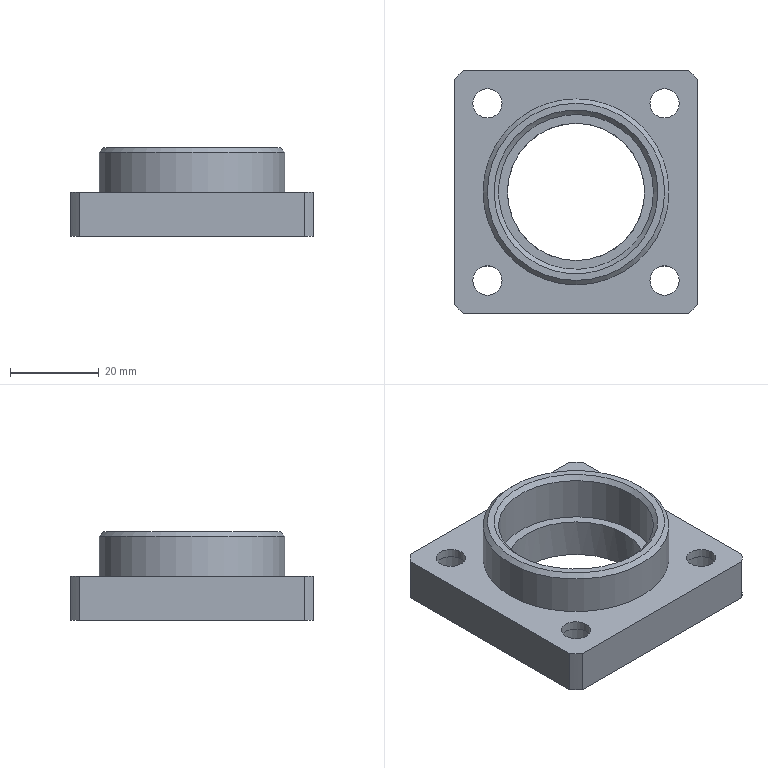Part | NX | 1 solid | 29 faces | box 55 x 55 x 20 mm | volume 23214 mm3 | cylinder 15 | plane 12 | cone 2 | commonest cylinder face diameters 6.6 x4 11 x4 75 x4 31 x1 35 x1 42 x1
STEP:
#1=CARTESIAN_POINT('',(16.7,20.,10.));
#2=VERTEX_POINT('',#1);
#3=CARTESIAN_POINT('',(20.,20.,10.));
#4=DIRECTION('',(0.,0.,-1.));
#5=DIRECTION('',(-1.,0.,0.));
#6=AXIS2_PLACEMENT_3D('',#3,#4,#5);
#7=CIRCLE('',#6,3.3);
#8=EDGE_CURVE('',#2,#2,#7,.T.);
#9=ORIENTED_EDGE('',*,*,#8,.T.);
#10=EDGE_LOOP('',(#9));
#11=FACE_BOUND('',#10,.T.);
#12=CARTESIAN_POINT('',(16.7,-20.,10.));
#13=VERTEX_POINT('',#12);
#14=CARTESIAN_POINT('',(20.,-20.,10.));
#15=DIRECTION('',(0.,0.,-1.));
#16=DIRECTION('',(-1.,0.,0.));
#17=AXIS2_PLACEMENT_3D('',#14,#15,#16);
#18=CIRCLE('',#17,3.3);
#19=EDGE_CURVE('',#13,#13,#18,.T.);
#20=ORIENTED_EDGE('',*,*,#19,.T.);
#21=EDGE_LOOP('',(#20));
#22=FACE_BOUND('',#21,.T.);
#23=CARTESIAN_POINT('',(-23.3,20.,10.));
#24=VERTEX_POINT('',#23);
#25=CARTESIAN_POINT('',(-20.,20.,10.));
#26=DIRECTION('',(0.,0.,-1.));
#27=DIRECTION('',(-1.,0.,0.));
#28=AXIS2_PLACEMENT_3D('',#25,#26,#27);
#29=CIRCLE('',#28,3.3);
#30=EDGE_CURVE('',#24,#24,#29,.T.);
#31=ORIENTED_EDGE('',*,*,#30,.T.);
#32=EDGE_LOOP('',(#31));
#33=FACE_BOUND('',#32,.T.);
#34=CARTESIAN_POINT('',(-23.3,-20.,10.));
#35=VERTEX_POINT('',#34);
#36=CARTESIAN_POINT('',(-20.,-20.,10.));
#37=DIRECTION('',(0.,0.,-1.));
#38=DIRECTION('',(-1.,0.,0.));
#39=AXIS2_PLACEMENT_3D('',#36,#37,#38);
#40=CIRCLE('',#39,3.3);
#41=EDGE_CURVE('',#35,#35,#40,.T.);
#42=ORIENTED_EDGE('',*,*,#41,.T.);
#43=EDGE_LOOP('',(#42));
#44=FACE_BOUND('',#43,.T.);
#45=CARTESIAN_POINT('',(-21.,0.,10.));
#46=VERTEX_POINT('',#45);
#47=CARTESIAN_POINT('',(0.,0.,10.));
#48=DIRECTION('',(0.,0.,-1.));
#49=DIRECTION('',(-1.,0.,0.));
#50=AXIS2_PLACEMENT_3D('',#47,#48,#49);
#51=CIRCLE('',#50,21.);
#52=EDGE_CURVE('',#46,#46,#51,.F.);
#53=ORIENTED_EDGE('',*,*,#52,.F.);
#54=EDGE_LOOP('',(#53));
#55=FACE_BOUND('',#54,.T.);
#56=CARTESIAN_POINT('',(-27.5,25.495,10.));
#57=VERTEX_POINT('',#56);
#58=CARTESIAN_POINT('',(-25.495,27.5,10.));
#59=VERTEX_POINT('',#58);
#60=CARTESIAN_POINT('',(0.,0.,10.));
#61=DIRECTION('',(0.,0.,-1.));
#62=DIRECTION('',(-1.,0.,0.));
#63=AXIS2_PLACEMENT_3D('',#60,#61,#62);
#64=CIRCLE('',#63,37.5);
#65=EDGE_CURVE('',#57,#59,#64,.T.);
#66=ORIENTED_EDGE('',*,*,#65,.F.);
#67=CARTESIAN_POINT('',(-27.5,-25.495,10.));
#68=VERTEX_POINT('',#67);
#69=CARTESIAN_POINT('',(-27.5,-27.5,10.));
#70=DIRECTION('',(0.,-1.,0.));
#71=VECTOR('',#70,1000.);
#72=LINE('',#69,#71);
#73=EDGE_CURVE('',#57,#68,#72,.T.);
#74=ORIENTED_EDGE('',*,*,#73,.T.);
#75=CARTESIAN_POINT('',(-25.495,-27.5,10.));
#76=VERTEX_POINT('',#75);
#77=CARTESIAN_POINT('',(0.,0.,10.));
#78=DIRECTION('',(0.,0.,-1.));
#79=DIRECTION('',(-1.,0.,0.));
#80=AXIS2_PLACEMENT_3D('',#77,#78,#79);
#81=CIRCLE('',#80,37.5);
#82=EDGE_CURVE('',#76,#68,#81,.T.);
#83=ORIENTED_EDGE('',*,*,#82,.F.);
#84=CARTESIAN_POINT('',(25.495,-27.5,10.));
#85=VERTEX_POINT('',#84);
#86=CARTESIAN_POINT('',(-27.5,-27.5,10.));
#87=DIRECTION('',(1.,0.,0.));
#88=VECTOR('',#87,1000.);
#89=LINE('',#86,#88);
#90=EDGE_CURVE('',#76,#85,#89,.T.);
#91=ORIENTED_EDGE('',*,*,#90,.T.);
#92=CARTESIAN_POINT('',(27.5,-25.495,10.));
#93=VERTEX_POINT('',#92);
#94=CARTESIAN_POINT('',(0.,0.,10.));
#95=DIRECTION('',(0.,0.,-1.));
#96=DIRECTION('',(-1.,0.,0.));
#97=AXIS2_PLACEMENT_3D('',#94,#95,#96);
#98=CIRCLE('',#97,37.5);
#99=EDGE_CURVE('',#93,#85,#98,.T.);
#100=ORIENTED_EDGE('',*,*,#99,.F.);
#101=CARTESIAN_POINT('',(27.5,25.495,10.));
#102=VERTEX_POINT('',#101);
#103=CARTESIAN_POINT('',(27.5,-27.5,10.));
#104=DIRECTION('',(0.,1.,0.));
#105=VECTOR('',#104,1000.);
#106=LINE('',#103,#105);
#107=EDGE_CURVE('',#93,#102,#106,.T.);
#108=ORIENTED_EDGE('',*,*,#107,.T.);
#109=CARTESIAN_POINT('',(25.495,27.5,10.));
#110=VERTEX_POINT('',#109);
#111=CARTESIAN_POINT('',(0.,0.,10.));
#112=DIRECTION('',(0.,0.,-1.));
#113=DIRECTION('',(-1.,0.,0.));
#114=AXIS2_PLACEMENT_3D('',#111,#112,#113);
#115=CIRCLE('',#114,37.5);
#116=EDGE_CURVE('',#110,#102,#115,.T.);
#117=ORIENTED_EDGE('',*,*,#116,.F.);
#118=CARTESIAN_POINT('',(-27.5,27.5,10.));
#119=DIRECTION('',(-1.,0.,0.));
#120=VECTOR('',#119,1000.);
#121=LINE('',#118,#120);
#122=EDGE_CURVE('',#110,#59,#121,.T.);
#123=ORIENTED_EDGE('',*,*,#122,.T.);
#124=EDGE_LOOP('',(#66,#74,#83,#91,#100,#108,#117,#123));
#125=FACE_BOUND('',#124,.T.);
#126=CARTESIAN_POINT('',(0.,0.,10.));
#127=DIRECTION('',(0.,0.,-1.));
#128=DIRECTION('',(-1.,0.,0.));
#129=AXIS2_PLACEMENT_3D('',#126,#127,#128);
#130=PLANE('',#129);
#131=ADVANCED_FACE('',(#11,#22,#33,#44,#55,#125),#130,.F.);
#132=CARTESIAN_POINT('',(27.5,25.495,0.));
#133=VERTEX_POINT('',#132);
#134=CARTESIAN_POINT('',(27.5,25.495,10.));
#135=DIRECTION('',(0.,0.,-1.));
#136=VECTOR('',#135,1000.);
#137=LINE('',#134,#136);
#138=EDGE_CURVE('',#102,#133,#137,.T.);
#139=ORIENTED_EDGE('',*,*,#138,.F.);
#140=ORIENTED_EDGE('',*,*,#107,.F.);
#141=CARTESIAN_POINT('',(27.5,-25.495,0.));
#142=VERTEX_POINT('',#141);
#143=CARTESIAN_POINT('',(27.5,-25.495,10.));
#144=DIRECTION('',(0.,0.,-1.));
#145=VECTOR('',#144,1000.);
#146=LINE('',#143,#145);
#147=EDGE_CURVE('',#142,#93,#146,.F.);
#148=ORIENTED_EDGE('',*,*,#147,.F.);
#149=CARTESIAN_POINT('',(27.5,-27.5,0.));
#150=DIRECTION('',(0.,1.,0.));
#151=VECTOR('',#150,1000.);
#152=LINE('',#149,#151);
#153=EDGE_CURVE('',#142,#133,#152,.T.);
#154=ORIENTED_EDGE('',*,*,#153,.T.);
#155=EDGE_LOOP('',(#139,#140,#148,#154));
#156=FACE_BOUND('',#155,.T.);
#157=CARTESIAN_POINT('',(27.5,-27.5,10.));
#158=DIRECTION('',(-1.,0.,0.));
#159=DIRECTION('',(0.,0.,1.));
#160=AXIS2_PLACEMENT_3D('',#157,#158,#159);
#161=PLANE('',#160);
#162=ADVANCED_FACE('',(#156),#161,.F.);
#163=CARTESIAN_POINT('',(-25.495,27.5,0.));
#164=VERTEX_POINT('',#163);
#165=CARTESIAN_POINT('',(-25.495,27.5,10.));
#166=DIRECTION('',(0.,0.,-1.));
#167=VECTOR('',#166,1000.);
#168=LINE('',#165,#167);
#169=EDGE_CURVE('',#59,#164,#168,.T.);
#170=ORIENTED_EDGE('',*,*,#169,.F.);
#171=ORIENTED_EDGE('',*,*,#122,.F.);
#172=CARTESIAN_POINT('',(25.495,27.5,0.));
#173=VERTEX_POINT('',#172);
#174=CARTESIAN_POINT('',(25.495,27.5,10.));
#175=DIRECTION('',(0.,0.,-1.));
#176=VECTOR('',#175,1000.);
#177=LINE('',#174,#176);
#178=EDGE_CURVE('',#173,#110,#177,.F.);
#179=ORIENTED_EDGE('',*,*,#178,.F.);
#180=CARTESIAN_POINT('',(-27.5,27.5,0.));
#181=DIRECTION('',(-1.,0.,0.));
#182=VECTOR('',#181,1000.);
#183=LINE('',#180,#182);
#184=EDGE_CURVE('',#173,#164,#183,.T.);
#185=ORIENTED_EDGE('',*,*,#184,.T.);
#186=EDGE_LOOP('',(#170,#171,#179,#185));
#187=FACE_BOUND('',#186,.T.);
#188=CARTESIAN_POINT('',(-27.5,27.5,10.));
#189=DIRECTION('',(0.,-1.,0.));
#190=DIRECTION('',(0.,0.,-1.));
#191=AXIS2_PLACEMENT_3D('',#188,#189,#190);
#192=PLANE('',#191);
#193=ADVANCED_FACE('',(#187),#192,.F.);
#194=CARTESIAN_POINT('',(-27.5,-25.495,0.));
#195=VERTEX_POINT('',#194);
#196=CARTESIAN_POINT('',(-27.5,-25.495,10.));
#197=DIRECTION('',(0.,0.,-1.));
#198=VECTOR('',#197,1000.);
#199=LINE('',#196,#198);
#200=EDGE_CURVE('',#68,#195,#199,.T.);
#201=ORIENTED_EDGE('',*,*,#200,.F.);
#202=ORIENTED_EDGE('',*,*,#73,.F.);
#203=CARTESIAN_POINT('',(-27.5,25.495,0.));
#204=VERTEX_POINT('',#203);
#205=CARTESIAN_POINT('',(-27.5,25.495,10.));
#206=DIRECTION('',(0.,0.,-1.));
#207=VECTOR('',#206,1000.);
#208=LINE('',#205,#207);
#209=EDGE_CURVE('',#204,#57,#208,.F.);
#210=ORIENTED_EDGE('',*,*,#209,.F.);
#211=CARTESIAN_POINT('',(-27.5,-27.5,0.));
#212=DIRECTION('',(0.,-1.,0.));
#213=VECTOR('',#212,1000.);
#214=LINE('',#211,#213);
#215=EDGE_CURVE('',#204,#195,#214,.T.);
#216=ORIENTED_EDGE('',*,*,#215,.T.);
#217=EDGE_LOOP('',(#201,#202,#210,#216));
#218=FACE_BOUND('',#217,.T.);
#219=CARTESIAN_POINT('',(-27.5,-27.5,10.));
#220=DIRECTION('',(1.,0.,0.));
#221=DIRECTION('',(0.,0.,-1.));
#222=AXIS2_PLACEMENT_3D('',#219,#220,#221);
#223=PLANE('',#222);
#224=ADVANCED_FACE('',(#218),#223,.F.);
#225=CARTESIAN_POINT('',(25.495,-27.5,0.));
#226=VERTEX_POINT('',#225);
#227=CARTESIAN_POINT('',(25.495,-27.5,10.));
#228=DIRECTION('',(0.,0.,-1.));
#229=VECTOR('',#228,1000.);
#230=LINE('',#227,#229);
#231=EDGE_CURVE('',#85,#226,#230,.T.);
#232=ORIENTED_EDGE('',*,*,#231,.F.);
#233=ORIENTED_EDGE('',*,*,#90,.F.);
#234=CARTESIAN_POINT('',(-25.495,-27.5,0.));
#235=VERTEX_POINT('',#234);
#236=CARTESIAN_POINT('',(-25.495,-27.5,10.));
#237=DIRECTION('',(0.,0.,-1.));
#238=VECTOR('',#237,1000.);
#239=LINE('',#236,#238);
#240=EDGE_CURVE('',#235,#76,#239,.F.);
#241=ORIENTED_EDGE('',*,*,#240,.F.);
#242=CARTESIAN_POINT('',(-27.5,-27.5,0.));
#243=DIRECTION('',(1.,0.,0.));
#244=VECTOR('',#243,1000.);
#245=LINE('',#242,#244);
#246=EDGE_CURVE('',#235,#226,#245,.T.);
#247=ORIENTED_EDGE('',*,*,#246,.T.);
#248=EDGE_LOOP('',(#232,#233,#241,#247));
#249=FACE_BOUND('',#248,.T.);
#250=CARTESIAN_POINT('',(-27.5,-27.5,10.));
#251=DIRECTION('',(0.,1.,0.));
#252=DIRECTION('',(0.,0.,1.));
#253=AXIS2_PLACEMENT_3D('',#250,#251,#252);
#254=PLANE('',#253);
#255=ADVANCED_FACE('',(#249),#254,.F.);
#256=CARTESIAN_POINT('',(14.5,20.,0.));
#257=VERTEX_POINT('',#256);
#258=CARTESIAN_POINT('',(20.,20.,0.));
#259=DIRECTION('',(0.,0.,-1.));
#260=DIRECTION('',(-1.,0.,0.));
#261=AXIS2_PLACEMENT_3D('',#258,#259,#260);
#262=CIRCLE('',#261,5.5);
#263=EDGE_CURVE('',#257,#257,#262,.T.);
#264=ORIENTED_EDGE('',*,*,#263,.F.);
#265=EDGE_LOOP('',(#264));
#266=FACE_BOUND('',#265,.T.);
#267=CARTESIAN_POINT('',(14.5,-20.,0.));
#268=VERTEX_POINT('',#267);
#269=CARTESIAN_POINT('',(20.,-20.,0.));
#270=DIRECTION('',(0.,0.,-1.));
#271=DIRECTION('',(-1.,0.,0.));
#272=AXIS2_PLACEMENT_3D('',#269,#270,#271);
#273=CIRCLE('',#272,5.5);
#274=EDGE_CURVE('',#268,#268,#273,.T.);
#275=ORIENTED_EDGE('',*,*,#274,.F.);
#276=EDGE_LOOP('',(#275));
#277=FACE_BOUND('',#276,.T.);
#278=CARTESIAN_POINT('',(-25.5,20.,0.));
#279=VERTEX_POINT('',#278);
#280=CARTESIAN_POINT('',(-20.,20.,0.));
#281=DIRECTION('',(0.,0.,-1.));
#282=DIRECTION('',(-1.,0.,0.));
#283=AXIS2_PLACEMENT_3D('',#280,#281,#282);
#284=CIRCLE('',#283,5.5);
#285=EDGE_CURVE('',#279,#279,#284,.T.);
#286=ORIENTED_EDGE('',*,*,#285,.F.);
#287=EDGE_LOOP('',(#286));
#288=FACE_BOUND('',#287,.T.);
#289=CARTESIAN_POINT('',(-25.5,-20.,0.));
#290=VERTEX_POINT('',#289);
#291=CARTESIAN_POINT('',(-20.,-20.,0.));
#292=DIRECTION('',(0.,0.,-1.));
#293=DIRECTION('',(-1.,0.,0.));
#294=AXIS2_PLACEMENT_3D('',#291,#292,#293);
#295=CIRCLE('',#294,5.5);
#296=EDGE_CURVE('',#290,#290,#295,.T.);
#297=ORIENTED_EDGE('',*,*,#296,.F.);
#298=EDGE_LOOP('',(#297));
#299=FACE_BOUND('',#298,.T.);
#300=CARTESIAN_POINT('',(-15.5,0.,0.));
#301=VERTEX_POINT('',#300);
#302=CARTESIAN_POINT('',(0.,0.,0.));
#303=DIRECTION('',(0.,0.,-1.));
#304=DIRECTION('',(-1.,0.,0.));
#305=AXIS2_PLACEMENT_3D('',#302,#303,#304);
#306=CIRCLE('',#305,15.5);
#307=EDGE_CURVE('',#301,#301,#306,.T.);
#308=ORIENTED_EDGE('',*,*,#307,.F.);
#309=EDGE_LOOP('',(#308));
#310=FACE_BOUND('',#309,.T.);
#311=ORIENTED_EDGE('',*,*,#215,.F.);
#312=CARTESIAN_POINT('',(0.,0.,0.));
#313=DIRECTION('',(0.,0.,-1.));
#314=DIRECTION('',(-1.,0.,0.));
#315=AXIS2_PLACEMENT_3D('',#312,#313,#314);
#316=CIRCLE('',#315,37.5);
#317=EDGE_CURVE('',#204,#164,#316,.T.);
#318=ORIENTED_EDGE('',*,*,#317,.T.);
#319=ORIENTED_EDGE('',*,*,#184,.F.);
#320=CARTESIAN_POINT('',(0.,0.,0.));
#321=DIRECTION('',(0.,0.,-1.));
#322=DIRECTION('',(-1.,0.,0.));
#323=AXIS2_PLACEMENT_3D('',#320,#321,#322);
#324=CIRCLE('',#323,37.5);
#325=EDGE_CURVE('',#173,#133,#324,.T.);
#326=ORIENTED_EDGE('',*,*,#325,.T.);
#327=ORIENTED_EDGE('',*,*,#153,.F.);
#328=CARTESIAN_POINT('',(0.,0.,0.));
#329=DIRECTION('',(0.,0.,-1.));
#330=DIRECTION('',(-1.,0.,0.));
#331=AXIS2_PLACEMENT_3D('',#328,#329,#330);
#332=CIRCLE('',#331,37.5);
#333=EDGE_CURVE('',#142,#226,#332,.T.);
#334=ORIENTED_EDGE('',*,*,#333,.T.);
#335=ORIENTED_EDGE('',*,*,#246,.F.);
#336=CARTESIAN_POINT('',(0.,0.,0.));
#337=DIRECTION('',(0.,0.,-1.));
#338=DIRECTION('',(-1.,0.,0.));
#339=AXIS2_PLACEMENT_3D('',#336,#337,#338);
#340=CIRCLE('',#339,37.5);
#341=EDGE_CURVE('',#235,#195,#340,.T.);
#342=ORIENTED_EDGE('',*,*,#341,.T.);
#343=EDGE_LOOP('',(#311,#318,#319,#326,#327,#334,#335,#342));
#344=FACE_BOUND('',#343,.T.);
#345=CARTESIAN_POINT('',(0.,0.,0.));
#346=DIRECTION('',(0.,0.,-1.));
#347=DIRECTION('',(-1.,0.,0.));
#348=AXIS2_PLACEMENT_3D('',#345,#346,#347);
#349=PLANE('',#348);
#350=ADVANCED_FACE('',(#266,#277,#288,#299,#310,#344),#349,.T.);
#351=CARTESIAN_POINT('',(21.,0.,19.));
#352=VERTEX_POINT('',#351);
#353=CARTESIAN_POINT('',(0.,0.,19.));
#354=DIRECTION('',(0.,0.,1.));
#355=DIRECTION('',(1.,0.,0.));
#356=AXIS2_PLACEMENT_3D('',#353,#354,#355);
#357=CIRCLE('',#356,21.);
#358=EDGE_CURVE('',#352,#352,#357,.F.);
#359=ORIENTED_EDGE('',*,*,#358,.T.);
#360=EDGE_LOOP('',(#359));
#361=FACE_BOUND('',#360,.T.);
#362=ORIENTED_EDGE('',*,*,#52,.T.);
#363=EDGE_LOOP('',(#362));
#364=FACE_BOUND('',#363,.T.);
#365=CARTESIAN_POINT('',(0.,0.,20.));
#366=DIRECTION('',(0.,0.,-1.));
#367=DIRECTION('',(-1.,0.,0.));
#368=AXIS2_PLACEMENT_3D('',#365,#366,#367);
#369=CYLINDRICAL_SURFACE('',#368,21.);
#370=ADVANCED_FACE('',(#361,#364),#369,.T.);
#371=CARTESIAN_POINT('',(18.5,0.,20.));
#372=VERTEX_POINT('',#371);
#373=CARTESIAN_POINT('',(0.,0.,20.));
#374=DIRECTION('',(0.,0.,1.));
#375=DIRECTION('',(1.,0.,0.));
#376=AXIS2_PLACEMENT_3D('',#373,#374,#375);
#377=CIRCLE('',#376,18.5);
#378=EDGE_CURVE('',#372,#372,#377,.F.);
#379=ORIENTED_EDGE('',*,*,#378,.T.);
#380=EDGE_LOOP('',(#379));
#381=FACE_BOUND('',#380,.T.);
#382=CARTESIAN_POINT('',(20.,0.,20.));
#383=VERTEX_POINT('',#382);
#384=CARTESIAN_POINT('',(0.,0.,20.));
#385=DIRECTION('',(0.,0.,1.));
#386=DIRECTION('',(1.,0.,0.));
#387=AXIS2_PLACEMENT_3D('',#384,#385,#386);
#388=CIRCLE('',#387,20.);
#389=EDGE_CURVE('',#383,#383,#388,.T.);
#390=ORIENTED_EDGE('',*,*,#389,.T.);
#391=EDGE_LOOP('',(#390));
#392=FACE_BOUND('',#391,.T.);
#393=CARTESIAN_POINT('',(0.,0.,20.));
#394=DIRECTION('',(0.,0.,1.));
#395=DIRECTION('',(1.,0.,0.));
#396=AXIS2_PLACEMENT_3D('',#393,#394,#395);
#397=PLANE('',#396);
#398=ADVANCED_FACE('',(#381,#392),#397,.T.);
#399=CARTESIAN_POINT('',(17.5,0.,19.));
#400=VERTEX_POINT('',#399);
#401=CARTESIAN_POINT('',(0.,0.,19.));
#402=DIRECTION('',(0.,0.,1.));
#403=DIRECTION('',(1.,0.,0.));
#404=AXIS2_PLACEMENT_3D('',#401,#402,#403);
#405=CIRCLE('',#404,17.5);
#406=EDGE_CURVE('',#400,#400,#405,.T.);
#407=ORIENTED_EDGE('',*,*,#406,.T.);
#408=EDGE_LOOP('',(#407));
#409=FACE_BOUND('',#408,.T.);
#410=CARTESIAN_POINT('',(17.5,0.,9.));
#411=VERTEX_POINT('',#410);
#412=CARTESIAN_POINT('',(0.,0.,9.));
#413=DIRECTION('',(0.,0.,1.));
#414=DIRECTION('',(1.,0.,0.));
#415=AXIS2_PLACEMENT_3D('',#412,#413,#414);
#416=CIRCLE('',#415,17.5);
#417=EDGE_CURVE('',#411,#411,#416,.T.);
#418=ORIENTED_EDGE('',*,*,#417,.F.);
#419=EDGE_LOOP('',(#418));
#420=FACE_BOUND('',#419,.T.);
#421=CARTESIAN_POINT('',(0.,0.,9.));
#422=DIRECTION('',(0.,0.,1.));
#423=DIRECTION('',(1.,0.,0.));
#424=AXIS2_PLACEMENT_3D('',#421,#422,#423);
#425=CYLINDRICAL_SURFACE('',#424,17.5);
#426=ADVANCED_FACE('',(#409,#420),#425,.F.);
#427=CARTESIAN_POINT('',(15.5,0.,9.));
#428=VERTEX_POINT('',#427);
#429=CARTESIAN_POINT('',(0.,0.,9.));
#430=DIRECTION('',(0.,0.,1.));
#431=DIRECTION('',(1.,0.,0.));
#432=AXIS2_PLACEMENT_3D('',#429,#430,#431);
#433=CIRCLE('',#432,15.5);
#434=EDGE_CURVE('',#428,#428,#433,.T.);
#435=ORIENTED_EDGE('',*,*,#434,.F.);
#436=EDGE_LOOP('',(#435));
#437=FACE_BOUND('',#436,.T.);
#438=ORIENTED_EDGE('',*,*,#417,.T.);
#439=EDGE_LOOP('',(#438));
#440=FACE_BOUND('',#439,.T.);
#441=CARTESIAN_POINT('',(0.,0.,9.));
#442=DIRECTION('',(0.,0.,1.));
#443=DIRECTION('',(1.,0.,0.));
#444=AXIS2_PLACEMENT_3D('',#441,#442,#443);
#445=PLANE('',#444);
#446=ADVANCED_FACE('',(#437,#440),#445,.T.);
#447=ORIENTED_EDGE('',*,*,#434,.T.);
#448=EDGE_LOOP('',(#447));
#449=FACE_BOUND('',#448,.T.);
#450=ORIENTED_EDGE('',*,*,#307,.T.);
#451=EDGE_LOOP('',(#450));
#452=FACE_BOUND('',#451,.T.);
#453=CARTESIAN_POINT('',(0.,0.,20.));
#454=DIRECTION('',(0.,0.,-1.));
#455=DIRECTION('',(-1.,0.,0.));
#456=AXIS2_PLACEMENT_3D('',#453,#454,#455);
#457=CYLINDRICAL_SURFACE('',#456,15.5);
#458=ADVANCED_FACE('',(#449,#452),#457,.F.);
#459=CARTESIAN_POINT('',(-23.3,-20.,8.));
#460=VERTEX_POINT('',#459);
#461=CARTESIAN_POINT('',(-20.,-20.,8.));
#462=DIRECTION('',(0.,0.,-1.));
#463=DIRECTION('',(-1.,0.,0.));
#464=AXIS2_PLACEMENT_3D('',#461,#462,#463);
#465=CIRCLE('',#464,3.3);
#466=EDGE_CURVE('',#460,#460,#465,.T.);
#467=ORIENTED_EDGE('',*,*,#466,.T.);
#468=EDGE_LOOP('',(#467));
#469=FACE_BOUND('',#468,.T.);
#470=ORIENTED_EDGE('',*,*,#41,.F.);
#471=EDGE_LOOP('',(#470));
#472=FACE_BOUND('',#471,.T.);
#473=CARTESIAN_POINT('',(-20.,-20.,0.));
#474=DIRECTION('',(0.,0.,-1.));
#475=DIRECTION('',(-1.,0.,0.));
#476=AXIS2_PLACEMENT_3D('',#473,#474,#475);
#477=CYLINDRICAL_SURFACE('',#476,3.3);
#478=ADVANCED_FACE('',(#469,#472),#477,.F.);
#479=ORIENTED_EDGE('',*,*,#466,.F.);
#480=EDGE_LOOP('',(#479));
#481=FACE_BOUND('',#480,.T.);
#482=CARTESIAN_POINT('',(-25.5,-20.,8.));
#483=VERTEX_POINT('',#482);
#484=CARTESIAN_POINT('',(-20.,-20.,8.));
#485=DIRECTION('',(0.,0.,-1.));
#486=DIRECTION('',(-1.,0.,0.));
#487=AXIS2_PLACEMENT_3D('',#484,#485,#486);
#488=CIRCLE('',#487,5.5);
#489=EDGE_CURVE('',#483,#483,#488,.T.);
#490=ORIENTED_EDGE('',*,*,#489,.T.);
#491=EDGE_LOOP('',(#490));
#492=FACE_BOUND('',#491,.T.);
#493=CARTESIAN_POINT('',(-16.7,-20.,8.));
#494=DIRECTION('',(0.,0.,1.));
#495=DIRECTION('',(1.,0.,0.));
#496=AXIS2_PLACEMENT_3D('',#493,#494,#495);
#497=PLANE('',#496);
#498=ADVANCED_FACE('',(#481,#492),#497,.F.);
#499=ORIENTED_EDGE('',*,*,#489,.F.);
#500=EDGE_LOOP('',(#499));
#501=FACE_BOUND('',#500,.T.);
#502=ORIENTED_EDGE('',*,*,#296,.T.);
#503=EDGE_LOOP('',(#502));
#504=FACE_BOUND('',#503,.T.);
#505=CARTESIAN_POINT('',(-20.,-20.,0.));
#506=DIRECTION('',(0.,0.,-1.));
#507=DIRECTION('',(-1.,0.,0.));
#508=AXIS2_PLACEMENT_3D('',#505,#506,#507);
#509=CYLINDRICAL_SURFACE('',#508,5.5);
#510=ADVANCED_FACE('',(#501,#504),#509,.F.);
#511=CARTESIAN_POINT('',(-23.3,20.,8.));
#512=VERTEX_POINT('',#511);
#513=CARTESIAN_POINT('',(-20.,20.,8.));
#514=DIRECTION('',(0.,0.,-1.));
#515=DIRECTION('',(-1.,0.,0.));
#516=AXIS2_PLACEMENT_3D('',#513,#514,#515);
#517=CIRCLE('',#516,3.3);
#518=EDGE_CURVE('',#512,#512,#517,.T.);
#519=ORIENTED_EDGE('',*,*,#518,.T.);
#520=EDGE_LOOP('',(#519));
#521=FACE_BOUND('',#520,.T.);
#522=ORIENTED_EDGE('',*,*,#30,.F.);
#523=EDGE_LOOP('',(#522));
#524=FACE_BOUND('',#523,.T.);
#525=CARTESIAN_POINT('',(-20.,20.,0.));
#526=DIRECTION('',(0.,0.,-1.));
#527=DIRECTION('',(-1.,0.,0.));
#528=AXIS2_PLACEMENT_3D('',#525,#526,#527);
#529=CYLINDRICAL_SURFACE('',#528,3.3);
#530=ADVANCED_FACE('',(#521,#524),#529,.F.);
#531=ORIENTED_EDGE('',*,*,#518,.F.);
#532=EDGE_LOOP('',(#531));
#533=FACE_BOUND('',#532,.T.);
#534=CARTESIAN_POINT('',(-25.5,20.,8.));
#535=VERTEX_POINT('',#534);
#536=CARTESIAN_POINT('',(-20.,20.,8.));
#537=DIRECTION('',(0.,0.,-1.));
#538=DIRECTION('',(-1.,0.,0.));
#539=AXIS2_PLACEMENT_3D('',#536,#537,#538);
#540=CIRCLE('',#539,5.5);
#541=EDGE_CURVE('',#535,#535,#540,.T.);
#542=ORIENTED_EDGE('',*,*,#541,.T.);
#543=EDGE_LOOP('',(#542));
#544=FACE_BOUND('',#543,.T.);
#545=CARTESIAN_POINT('',(-16.7,20.,8.));
#546=DIRECTION('',(0.,0.,1.));
#547=DIRECTION('',(1.,0.,0.));
#548=AXIS2_PLACEMENT_3D('',#545,#546,#547);
#549=PLANE('',#548);
#550=ADVANCED_FACE('',(#533,#544),#549,.F.);
#551=ORIENTED_EDGE('',*,*,#541,.F.);
#552=EDGE_LOOP('',(#551));
#553=FACE_BOUND('',#552,.T.);
#554=ORIENTED_EDGE('',*,*,#285,.T.);
#555=EDGE_LOOP('',(#554));
#556=FACE_BOUND('',#555,.T.);
#557=CARTESIAN_POINT('',(-20.,20.,0.));
#558=DIRECTION('',(0.,0.,-1.));
#559=DIRECTION('',(-1.,0.,0.));
#560=AXIS2_PLACEMENT_3D('',#557,#558,#559);
#561=CYLINDRICAL_SURFACE('',#560,5.5);
#562=ADVANCED_FACE('',(#553,#556),#561,.F.);
#563=CARTESIAN_POINT('',(16.7,-20.,8.));
#564=VERTEX_POINT('',#563);
#565=CARTESIAN_POINT('',(20.,-20.,8.));
#566=DIRECTION('',(0.,0.,-1.));
#567=DIRECTION('',(-1.,0.,0.));
#568=AXIS2_PLACEMENT_3D('',#565,#566,#567);
#569=CIRCLE('',#568,3.3);
#570=EDGE_CURVE('',#564,#564,#569,.T.);
#571=ORIENTED_EDGE('',*,*,#570,.T.);
#572=EDGE_LOOP('',(#571));
#573=FACE_BOUND('',#572,.T.);
#574=ORIENTED_EDGE('',*,*,#19,.F.);
#575=EDGE_LOOP('',(#574));
#576=FACE_BOUND('',#575,.T.);
#577=CARTESIAN_POINT('',(20.,-20.,0.));
#578=DIRECTION('',(0.,0.,-1.));
#579=DIRECTION('',(-1.,0.,0.));
#580=AXIS2_PLACEMENT_3D('',#577,#578,#579);
#581=CYLINDRICAL_SURFACE('',#580,3.3);
#582=ADVANCED_FACE('',(#573,#576),#581,.F.);
#583=ORIENTED_EDGE('',*,*,#570,.F.);
#584=EDGE_LOOP('',(#583));
#585=FACE_BOUND('',#584,.T.);
#586=CARTESIAN_POINT('',(14.5,-20.,8.));
#587=VERTEX_POINT('',#586);
#588=CARTESIAN_POINT('',(20.,-20.,8.));
#589=DIRECTION('',(0.,0.,-1.));
#590=DIRECTION('',(-1.,0.,0.));
#591=AXIS2_PLACEMENT_3D('',#588,#589,#590);
#592=CIRCLE('',#591,5.5);
#593=EDGE_CURVE('',#587,#587,#592,.T.);
#594=ORIENTED_EDGE('',*,*,#593,.T.);
#595=EDGE_LOOP('',(#594));
#596=FACE_BOUND('',#595,.T.);
#597=CARTESIAN_POINT('',(23.3,-20.,8.));
#598=DIRECTION('',(0.,0.,1.));
#599=DIRECTION('',(1.,0.,0.));
#600=AXIS2_PLACEMENT_3D('',#597,#598,#599);
#601=PLANE('',#600);
#602=ADVANCED_FACE('',(#585,#596),#601,.F.);
#603=ORIENTED_EDGE('',*,*,#593,.F.);
#604=EDGE_LOOP('',(#603));
#605=FACE_BOUND('',#604,.T.);
#606=ORIENTED_EDGE('',*,*,#274,.T.);
#607=EDGE_LOOP('',(#606));
#608=FACE_BOUND('',#607,.T.);
#609=CARTESIAN_POINT('',(20.,-20.,0.));
#610=DIRECTION('',(0.,0.,-1.));
#611=DIRECTION('',(-1.,0.,0.));
#612=AXIS2_PLACEMENT_3D('',#609,#610,#611);
#613=CYLINDRICAL_SURFACE('',#612,5.5);
#614=ADVANCED_FACE('',(#605,#608),#613,.F.);
#615=CARTESIAN_POINT('',(16.7,20.,8.));
#616=VERTEX_POINT('',#615);
#617=CARTESIAN_POINT('',(20.,20.,8.));
#618=DIRECTION('',(0.,0.,-1.));
#619=DIRECTION('',(-1.,0.,0.));
#620=AXIS2_PLACEMENT_3D('',#617,#618,#619);
#621=CIRCLE('',#620,3.3);
#622=EDGE_CURVE('',#616,#616,#621,.T.);
#623=ORIENTED_EDGE('',*,*,#622,.T.);
#624=EDGE_LOOP('',(#623));
#625=FACE_BOUND('',#624,.T.);
#626=ORIENTED_EDGE('',*,*,#8,.F.);
#627=EDGE_LOOP('',(#626));
#628=FACE_BOUND('',#627,.T.);
#629=CARTESIAN_POINT('',(20.,20.,0.));
#630=DIRECTION('',(0.,0.,-1.));
#631=DIRECTION('',(-1.,0.,0.));
#632=AXIS2_PLACEMENT_3D('',#629,#630,#631);
#633=CYLINDRICAL_SURFACE('',#632,3.3);
#634=ADVANCED_FACE('',(#625,#628),#633,.F.);
#635=ORIENTED_EDGE('',*,*,#622,.F.);
#636=EDGE_LOOP('',(#635));
#637=FACE_BOUND('',#636,.T.);
#638=CARTESIAN_POINT('',(14.5,20.,8.));
#639=VERTEX_POINT('',#638);
#640=CARTESIAN_POINT('',(20.,20.,8.));
#641=DIRECTION('',(0.,0.,-1.));
#642=DIRECTION('',(-1.,0.,0.));
#643=AXIS2_PLACEMENT_3D('',#640,#641,#642);
#644=CIRCLE('',#643,5.5);
#645=EDGE_CURVE('',#639,#639,#644,.T.);
#646=ORIENTED_EDGE('',*,*,#645,.T.);
#647=EDGE_LOOP('',(#646));
#648=FACE_BOUND('',#647,.T.);
#649=CARTESIAN_POINT('',(23.3,20.,8.));
#650=DIRECTION('',(0.,0.,1.));
#651=DIRECTION('',(1.,0.,0.));
#652=AXIS2_PLACEMENT_3D('',#649,#650,#651);
#653=PLANE('',#652);
#654=ADVANCED_FACE('',(#637,#648),#653,.F.);
#655=ORIENTED_EDGE('',*,*,#645,.F.);
#656=EDGE_LOOP('',(#655));
#657=FACE_BOUND('',#656,.T.);
#658=ORIENTED_EDGE('',*,*,#263,.T.);
#659=EDGE_LOOP('',(#658));
#660=FACE_BOUND('',#659,.T.);
#661=CARTESIAN_POINT('',(20.,20.,0.));
#662=DIRECTION('',(0.,0.,-1.));
#663=DIRECTION('',(-1.,0.,0.));
#664=AXIS2_PLACEMENT_3D('',#661,#662,#663);
#665=CYLINDRICAL_SURFACE('',#664,5.5);
#666=ADVANCED_FACE('',(#657,#660),#665,.F.);
#667=ORIENTED_EDGE('',*,*,#378,.F.);
#668=EDGE_LOOP('',(#667));
#669=FACE_BOUND('',#668,.T.);
#670=ORIENTED_EDGE('',*,*,#406,.F.);
#671=EDGE_LOOP('',(#670));
#672=FACE_BOUND('',#671,.T.);
#673=CARTESIAN_POINT('',(0.,0.,19.));
#674=DIRECTION('',(0.,0.,1.));
#675=DIRECTION('',(1.,0.,0.));
#676=AXIS2_PLACEMENT_3D('',#673,#674,#675);
#677=CONICAL_SURFACE('',#676,17.5,0.7854);
#678=ADVANCED_FACE('',(#669,#672),#677,.F.);
#679=ORIENTED_EDGE('',*,*,#358,.F.);
#680=EDGE_LOOP('',(#679));
#681=FACE_BOUND('',#680,.T.);
#682=ORIENTED_EDGE('',*,*,#389,.F.);
#683=EDGE_LOOP('',(#682));
#684=FACE_BOUND('',#683,.T.);
#685=CARTESIAN_POINT('',(0.,0.,20.));
#686=DIRECTION('',(0.,0.,-1.));
#687=DIRECTION('',(-1.,0.,0.));
#688=AXIS2_PLACEMENT_3D('',#685,#686,#687);
#689=CONICAL_SURFACE('',#688,20.,0.7854);
#690=ADVANCED_FACE('',(#681,#684),#689,.T.);
#691=ORIENTED_EDGE('',*,*,#200,.T.);
#692=ORIENTED_EDGE('',*,*,#341,.F.);
#693=ORIENTED_EDGE('',*,*,#240,.T.);
#694=ORIENTED_EDGE('',*,*,#82,.T.);
#695=EDGE_LOOP('',(#691,#692,#693,#694));
#696=FACE_BOUND('',#695,.T.);
#697=CARTESIAN_POINT('',(0.,0.,10.));
#698=DIRECTION('',(0.,0.,-1.));
#699=DIRECTION('',(-1.,0.,0.));
#700=AXIS2_PLACEMENT_3D('',#697,#698,#699);
#701=CYLINDRICAL_SURFACE('',#700,37.5);
#702=ADVANCED_FACE('',(#696),#701,.T.);
#703=ORIENTED_EDGE('',*,*,#147,.T.);
#704=ORIENTED_EDGE('',*,*,#99,.T.);
#705=ORIENTED_EDGE('',*,*,#231,.T.);
#706=ORIENTED_EDGE('',*,*,#333,.F.);
#707=EDGE_LOOP('',(#703,#704,#705,#706));
#708=FACE_BOUND('',#707,.T.);
#709=CARTESIAN_POINT('',(0.,0.,10.));
#710=DIRECTION('',(0.,0.,-1.));
#711=DIRECTION('',(-1.,0.,0.));
#712=AXIS2_PLACEMENT_3D('',#709,#710,#711);
#713=CYLINDRICAL_SURFACE('',#712,37.5);
#714=ADVANCED_FACE('',(#708),#713,.T.);
#715=ORIENTED_EDGE('',*,*,#138,.T.);
#716=ORIENTED_EDGE('',*,*,#325,.F.);
#717=ORIENTED_EDGE('',*,*,#178,.T.);
#718=ORIENTED_EDGE('',*,*,#116,.T.);
#719=EDGE_LOOP('',(#715,#716,#717,#718));
#720=FACE_BOUND('',#719,.T.);
#721=CARTESIAN_POINT('',(0.,0.,10.));
#722=DIRECTION('',(0.,0.,-1.));
#723=DIRECTION('',(-1.,0.,0.));
#724=AXIS2_PLACEMENT_3D('',#721,#722,#723);
#725=CYLINDRICAL_SURFACE('',#724,37.5);
#726=ADVANCED_FACE('',(#720),#725,.T.);
#727=ORIENTED_EDGE('',*,*,#169,.T.);
#728=ORIENTED_EDGE('',*,*,#317,.F.);
#729=ORIENTED_EDGE('',*,*,#209,.T.);
#730=ORIENTED_EDGE('',*,*,#65,.T.);
#731=EDGE_LOOP('',(#727,#728,#729,#730));
#732=FACE_BOUND('',#731,.T.);
#733=CARTESIAN_POINT('',(0.,0.,10.));
#734=DIRECTION('',(0.,0.,-1.));
#735=DIRECTION('',(-1.,0.,0.));
#736=AXIS2_PLACEMENT_3D('',#733,#734,#735);
#737=CYLINDRICAL_SURFACE('',#736,37.5);
#738=ADVANCED_FACE('',(#732),#737,.T.);
#739=CLOSED_SHELL('',(#131,#162,#193,#224,#255,#350,#370,#398,#426,#446,#458,#478,#498,#510,#530,#550,#562,#582,#602,#614,#634,#654,#666,#678,#690,#702,#714,#726,#738));
#740=MANIFOLD_SOLID_BREP('',#739);
#741=(LENGTH_UNIT()NAMED_UNIT(*)SI_UNIT(.MILLI.,.METRE.));
#742=UNCERTAINTY_MEASURE_WITH_UNIT(LENGTH_MEASURE(0.00001),#741,'','');
#743=(NAMED_UNIT(*)PLANE_ANGLE_UNIT()SI_UNIT($,.RADIAN.));
#744=(NAMED_UNIT(*)SI_UNIT($,.STERADIAN.)SOLID_ANGLE_UNIT());
#745=(GEOMETRIC_REPRESENTATION_CONTEXT(3)GLOBAL_UNCERTAINTY_ASSIGNED_CONTEXT((#742))GLOBAL_UNIT_ASSIGNED_CONTEXT((#741,#743,#744))REPRESENTATION_CONTEXT('',''));
#746=ADVANCED_BREP_SHAPE_REPRESENTATION('',(#740),#745);